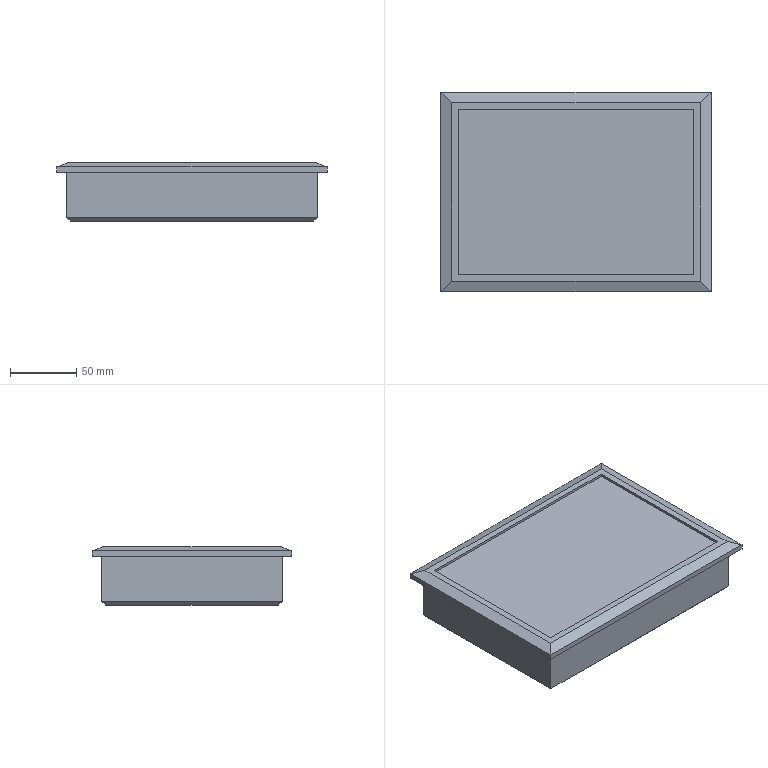Part | STEP file | Xinje TH765 touch screen | 1 solid | 24 faces | box 204 x 150.5 x 44 mm | volume 1119032 mm3 | plane 24
STEP:
#1=CARTESIAN_POINT('',(0.,0.,0.));
#2=DIRECTION('',(0.,0.,1.));
#3=DIRECTION('',(1.,0.,0.));
#4=AXIS2_PLACEMENT_3D('',#1,#2,#3);
#5=CARTESIAN_POINT('',(-43.829,26.896,37.));
#6=VERTEX_POINT('',#5);
#7=CARTESIAN_POINT('',(-43.829,26.896,3.));
#8=VERTEX_POINT('',#7);
#9=CARTESIAN_POINT('',(-43.829,26.896,37.));
#10=DIRECTION('',(0.,0.,-1.));
#11=VECTOR('',#10,1.);
#12=LINE('',#9,#11);
#13=CARTESIAN_POINT('',(-43.829,-109.604,37.));
#14=DIRECTION('',(1.,0.,0.));
#15=DIRECTION('',(0.,0.,-1.));
#16=AXIS2_PLACEMENT_3D('',#13,#14,#15);
#17=PLANE('',#16);
#18=CARTESIAN_POINT('',(0.,136.5));
#19=DIRECTION('',(1.,0.));
#20=VECTOR('',#19,1.);
#21=LINE('',#18,#20);
#22=(GEOMETRIC_REPRESENTATION_CONTEXT(2)PARAMETRIC_REPRESENTATION_CONTEXT()REPRESENTATION_CONTEXT('',''));
#23=DEFINITIONAL_REPRESENTATION('',(#21),#22);
#24=PCURVE('',#17,#23);
#25=CARTESIAN_POINT('',(-43.829,26.896,37.));
#26=DIRECTION('',(0.,-1.,0.));
#27=DIRECTION('',(0.,0.,-1.));
#28=AXIS2_PLACEMENT_3D('',#25,#26,#27);
#29=PLANE('',#28);
#30=CARTESIAN_POINT('',(0.,0.));
#31=DIRECTION('',(1.,0.));
#32=VECTOR('',#31,1.);
#33=LINE('',#30,#32);
#34=(GEOMETRIC_REPRESENTATION_CONTEXT(2)PARAMETRIC_REPRESENTATION_CONTEXT()REPRESENTATION_CONTEXT('',''));
#35=DEFINITIONAL_REPRESENTATION('',(#33),#34);
#36=PCURVE('',#29,#35);
#37=SURFACE_CURVE('',#12,(#24,#36),.PCURVE_S1.);
#38=EDGE_CURVE('',#6,#8,#37,.T.);
#39=ORIENTED_EDGE('',*,*,#38,.T.);
#40=CARTESIAN_POINT('',(-43.829,-109.604,3.));
#41=VERTEX_POINT('',#40);
#42=CARTESIAN_POINT('',(-43.829,-109.604,3.));
#43=DIRECTION('',(0.,-1.,0.));
#44=VECTOR('',#43,1.);
#45=LINE('',#42,#44);
#46=CARTESIAN_POINT('',(34.,0.));
#47=DIRECTION('',(0.,-1.));
#48=VECTOR('',#47,1.);
#49=LINE('',#46,#48);
#50=(GEOMETRIC_REPRESENTATION_CONTEXT(2)PARAMETRIC_REPRESENTATION_CONTEXT()REPRESENTATION_CONTEXT('',''));
#51=DEFINITIONAL_REPRESENTATION('',(#49),#50);
#52=PCURVE('',#17,#51);
#53=CARTESIAN_POINT('',(-43.829,-109.604,3.));
#54=DIRECTION('',(-0.7071,0.,-0.7071));
#55=DIRECTION('',(0.,1.,0.));
#56=AXIS2_PLACEMENT_3D('',#53,#54,#55);
#57=PLANE('',#56);
#58=CARTESIAN_POINT('',(0.,0.));
#59=DIRECTION('',(-1.,0.));
#60=VECTOR('',#59,1.);
#61=LINE('',#58,#60);
#62=(GEOMETRIC_REPRESENTATION_CONTEXT(2)PARAMETRIC_REPRESENTATION_CONTEXT()REPRESENTATION_CONTEXT('',''));
#63=DEFINITIONAL_REPRESENTATION('',(#61),#62);
#64=PCURVE('',#57,#63);
#65=SURFACE_CURVE('',#45,(#52,#64),.PCURVE_S1.);
#66=EDGE_CURVE('',#8,#41,#65,.T.);
#67=ORIENTED_EDGE('',*,*,#66,.T.);
#68=CARTESIAN_POINT('',(-43.829,-109.604,37.));
#69=VERTEX_POINT('',#68);
#70=CARTESIAN_POINT('',(-43.829,-109.604,37.));
#71=DIRECTION('',(0.,0.,-1.));
#72=VECTOR('',#71,1.);
#73=LINE('',#70,#72);
#74=CARTESIAN_POINT('',(0.,0.));
#75=DIRECTION('',(1.,0.));
#76=VECTOR('',#75,1.);
#77=LINE('',#74,#76);
#78=(GEOMETRIC_REPRESENTATION_CONTEXT(2)PARAMETRIC_REPRESENTATION_CONTEXT()REPRESENTATION_CONTEXT('',''));
#79=DEFINITIONAL_REPRESENTATION('',(#77),#78);
#80=PCURVE('',#17,#79);
#81=CARTESIAN_POINT('',(-43.829,-109.604,37.));
#82=DIRECTION('',(0.,1.,0.));
#83=DIRECTION('',(0.,0.,1.));
#84=AXIS2_PLACEMENT_3D('',#81,#82,#83);
#85=PLANE('',#84);
#86=CARTESIAN_POINT('',(0.,0.));
#87=DIRECTION('',(-1.,0.));
#88=VECTOR('',#87,1.);
#89=LINE('',#86,#88);
#90=(GEOMETRIC_REPRESENTATION_CONTEXT(2)PARAMETRIC_REPRESENTATION_CONTEXT()REPRESENTATION_CONTEXT('',''));
#91=DEFINITIONAL_REPRESENTATION('',(#89),#90);
#92=PCURVE('',#85,#91);
#93=SURFACE_CURVE('',#73,(#80,#92),.PCURVE_S1.);
#94=EDGE_CURVE('',#69,#41,#93,.T.);
#95=ORIENTED_EDGE('',*,*,#94,.F.);
#96=CARTESIAN_POINT('',(-43.829,-109.604,37.));
#97=DIRECTION('',(0.,-1.,0.));
#98=VECTOR('',#97,1.);
#99=LINE('',#96,#98);
#100=CARTESIAN_POINT('',(0.,0.));
#101=DIRECTION('',(0.,-1.));
#102=VECTOR('',#101,1.);
#103=LINE('',#100,#102);
#104=(GEOMETRIC_REPRESENTATION_CONTEXT(2)PARAMETRIC_REPRESENTATION_CONTEXT()REPRESENTATION_CONTEXT('',''));
#105=DEFINITIONAL_REPRESENTATION('',(#103),#104);
#106=PCURVE('',#17,#105);
#107=CARTESIAN_POINT('',(0.,0.,37.));
#108=DIRECTION('',(0.,0.,-1.));
#109=DIRECTION('',(-1.,0.,0.));
#110=AXIS2_PLACEMENT_3D('',#107,#108,#109);
#111=PLANE('',#110);
#112=CARTESIAN_POINT('',(43.829,-109.604));
#113=DIRECTION('',(0.,-1.));
#114=VECTOR('',#113,1.);
#115=LINE('',#112,#114);
#116=(GEOMETRIC_REPRESENTATION_CONTEXT(2)PARAMETRIC_REPRESENTATION_CONTEXT()REPRESENTATION_CONTEXT('',''));
#117=DEFINITIONAL_REPRESENTATION('',(#115),#116);
#118=PCURVE('',#111,#117);
#119=SURFACE_CURVE('',#99,(#106,#118),.PCURVE_S1.);
#120=EDGE_CURVE('',#6,#69,#119,.T.);
#121=ORIENTED_EDGE('',*,*,#120,.F.);
#122=EDGE_LOOP('',(#39,#67,#95,#121));
#123=FACE_BOUND('',#122,.T.);
#124=ADVANCED_FACE('',(#123),#17,.F.);
#125=ORIENTED_EDGE('',*,*,#94,.T.);
#126=CARTESIAN_POINT('',(146.171,-109.604,3.));
#127=VERTEX_POINT('',#126);
#128=CARTESIAN_POINT('',(146.171,-109.604,3.));
#129=DIRECTION('',(1.,0.,0.));
#130=VECTOR('',#129,1.);
#131=LINE('',#128,#130);
#132=CARTESIAN_POINT('',(-34.,190.));
#133=DIRECTION('',(0.,1.));
#134=VECTOR('',#133,1.);
#135=LINE('',#132,#134);
#136=(GEOMETRIC_REPRESENTATION_CONTEXT(2)PARAMETRIC_REPRESENTATION_CONTEXT()REPRESENTATION_CONTEXT('',''));
#137=DEFINITIONAL_REPRESENTATION('',(#135),#136);
#138=PCURVE('',#85,#137);
#139=CARTESIAN_POINT('',(-43.829,-109.604,3.));
#140=DIRECTION('',(0.,-0.7071,-0.7071));
#141=DIRECTION('',(-1.,0.,0.));
#142=AXIS2_PLACEMENT_3D('',#139,#140,#141);
#143=PLANE('',#142);
#144=CARTESIAN_POINT('',(-190.,0.));
#145=DIRECTION('',(-1.,0.));
#146=VECTOR('',#145,1.);
#147=LINE('',#144,#146);
#148=(GEOMETRIC_REPRESENTATION_CONTEXT(2)PARAMETRIC_REPRESENTATION_CONTEXT()REPRESENTATION_CONTEXT('',''));
#149=DEFINITIONAL_REPRESENTATION('',(#147),#148);
#150=PCURVE('',#143,#149);
#151=SURFACE_CURVE('',#131,(#138,#150),.PCURVE_S1.);
#152=EDGE_CURVE('',#41,#127,#151,.T.);
#153=ORIENTED_EDGE('',*,*,#152,.T.);
#154=CARTESIAN_POINT('',(146.171,-109.604,37.));
#155=VERTEX_POINT('',#154);
#156=CARTESIAN_POINT('',(146.171,-109.604,37.));
#157=DIRECTION('',(0.,0.,-1.));
#158=VECTOR('',#157,1.);
#159=LINE('',#156,#158);
#160=CARTESIAN_POINT('',(0.,190.));
#161=DIRECTION('',(-1.,0.));
#162=VECTOR('',#161,1.);
#163=LINE('',#160,#162);
#164=(GEOMETRIC_REPRESENTATION_CONTEXT(2)PARAMETRIC_REPRESENTATION_CONTEXT()REPRESENTATION_CONTEXT('',''));
#165=DEFINITIONAL_REPRESENTATION('',(#163),#164);
#166=PCURVE('',#85,#165);
#167=CARTESIAN_POINT('',(146.171,-109.604,37.));
#168=DIRECTION('',(-1.,0.,0.));
#169=DIRECTION('',(0.,0.,1.));
#170=AXIS2_PLACEMENT_3D('',#167,#168,#169);
#171=PLANE('',#170);
#172=CARTESIAN_POINT('',(0.,0.));
#173=DIRECTION('',(-1.,0.));
#174=VECTOR('',#173,1.);
#175=LINE('',#172,#174);
#176=(GEOMETRIC_REPRESENTATION_CONTEXT(2)PARAMETRIC_REPRESENTATION_CONTEXT()REPRESENTATION_CONTEXT('',''));
#177=DEFINITIONAL_REPRESENTATION('',(#175),#176);
#178=PCURVE('',#171,#177);
#179=SURFACE_CURVE('',#159,(#166,#178),.PCURVE_S1.);
#180=EDGE_CURVE('',#155,#127,#179,.T.);
#181=ORIENTED_EDGE('',*,*,#180,.F.);
#182=CARTESIAN_POINT('',(-43.829,-109.604,37.));
#183=DIRECTION('',(1.,0.,0.));
#184=VECTOR('',#183,1.);
#185=LINE('',#182,#184);
#186=CARTESIAN_POINT('',(0.,0.));
#187=DIRECTION('',(0.,1.));
#188=VECTOR('',#187,1.);
#189=LINE('',#186,#188);
#190=(GEOMETRIC_REPRESENTATION_CONTEXT(2)PARAMETRIC_REPRESENTATION_CONTEXT()REPRESENTATION_CONTEXT('',''));
#191=DEFINITIONAL_REPRESENTATION('',(#189),#190);
#192=PCURVE('',#85,#191);
#193=CARTESIAN_POINT('',(43.829,-109.604));
#194=DIRECTION('',(-1.,0.));
#195=VECTOR('',#194,1.);
#196=LINE('',#193,#195);
#197=(GEOMETRIC_REPRESENTATION_CONTEXT(2)PARAMETRIC_REPRESENTATION_CONTEXT()REPRESENTATION_CONTEXT('',''));
#198=DEFINITIONAL_REPRESENTATION('',(#196),#197);
#199=PCURVE('',#111,#198);
#200=SURFACE_CURVE('',#185,(#192,#199),.PCURVE_S1.);
#201=EDGE_CURVE('',#69,#155,#200,.T.);
#202=ORIENTED_EDGE('',*,*,#201,.F.);
#203=EDGE_LOOP('',(#125,#153,#181,#202));
#204=FACE_BOUND('',#203,.T.);
#205=ADVANCED_FACE('',(#204),#85,.F.);
#206=ORIENTED_EDGE('',*,*,#180,.T.);
#207=CARTESIAN_POINT('',(146.171,26.896,3.));
#208=VERTEX_POINT('',#207);
#209=CARTESIAN_POINT('',(146.171,26.896,3.));
#210=DIRECTION('',(0.,1.,0.));
#211=VECTOR('',#210,1.);
#212=LINE('',#209,#211);
#213=CARTESIAN_POINT('',(-34.,136.5));
#214=DIRECTION('',(0.,1.));
#215=VECTOR('',#214,1.);
#216=LINE('',#213,#215);
#217=(GEOMETRIC_REPRESENTATION_CONTEXT(2)PARAMETRIC_REPRESENTATION_CONTEXT()REPRESENTATION_CONTEXT('',''));
#218=DEFINITIONAL_REPRESENTATION('',(#216),#217);
#219=PCURVE('',#171,#218);
#220=CARTESIAN_POINT('',(146.171,-109.604,3.));
#221=DIRECTION('',(0.7071,0.,-0.7071));
#222=DIRECTION('',(0.,-1.,0.));
#223=AXIS2_PLACEMENT_3D('',#220,#221,#222);
#224=PLANE('',#223);
#225=CARTESIAN_POINT('',(-136.5,0.));
#226=DIRECTION('',(-1.,0.));
#227=VECTOR('',#226,1.);
#228=LINE('',#225,#227);
#229=(GEOMETRIC_REPRESENTATION_CONTEXT(2)PARAMETRIC_REPRESENTATION_CONTEXT()REPRESENTATION_CONTEXT('',''));
#230=DEFINITIONAL_REPRESENTATION('',(#228),#229);
#231=PCURVE('',#224,#230);
#232=SURFACE_CURVE('',#212,(#219,#231),.PCURVE_S1.);
#233=EDGE_CURVE('',#127,#208,#232,.T.);
#234=ORIENTED_EDGE('',*,*,#233,.T.);
#235=CARTESIAN_POINT('',(146.171,26.896,37.));
#236=VERTEX_POINT('',#235);
#237=CARTESIAN_POINT('',(146.171,26.896,37.));
#238=DIRECTION('',(0.,0.,-1.));
#239=VECTOR('',#238,1.);
#240=LINE('',#237,#239);
#241=CARTESIAN_POINT('',(0.,136.5));
#242=DIRECTION('',(-1.,0.));
#243=VECTOR('',#242,1.);
#244=LINE('',#241,#243);
#245=(GEOMETRIC_REPRESENTATION_CONTEXT(2)PARAMETRIC_REPRESENTATION_CONTEXT()REPRESENTATION_CONTEXT('',''));
#246=DEFINITIONAL_REPRESENTATION('',(#244),#245);
#247=PCURVE('',#171,#246);
#248=CARTESIAN_POINT('',(0.,190.));
#249=DIRECTION('',(1.,0.));
#250=VECTOR('',#249,1.);
#251=LINE('',#248,#250);
#252=(GEOMETRIC_REPRESENTATION_CONTEXT(2)PARAMETRIC_REPRESENTATION_CONTEXT()REPRESENTATION_CONTEXT('',''));
#253=DEFINITIONAL_REPRESENTATION('',(#251),#252);
#254=PCURVE('',#29,#253);
#255=SURFACE_CURVE('',#240,(#247,#254),.PCURVE_S1.);
#256=EDGE_CURVE('',#236,#208,#255,.T.);
#257=ORIENTED_EDGE('',*,*,#256,.F.);
#258=CARTESIAN_POINT('',(146.171,-109.604,37.));
#259=DIRECTION('',(0.,1.,0.));
#260=VECTOR('',#259,1.);
#261=LINE('',#258,#260);
#262=CARTESIAN_POINT('',(0.,0.));
#263=DIRECTION('',(0.,1.));
#264=VECTOR('',#263,1.);
#265=LINE('',#262,#264);
#266=(GEOMETRIC_REPRESENTATION_CONTEXT(2)PARAMETRIC_REPRESENTATION_CONTEXT()REPRESENTATION_CONTEXT('',''));
#267=DEFINITIONAL_REPRESENTATION('',(#265),#266);
#268=PCURVE('',#171,#267);
#269=CARTESIAN_POINT('',(-146.171,-109.604));
#270=DIRECTION('',(0.,1.));
#271=VECTOR('',#270,1.);
#272=LINE('',#269,#271);
#273=(GEOMETRIC_REPRESENTATION_CONTEXT(2)PARAMETRIC_REPRESENTATION_CONTEXT()REPRESENTATION_CONTEXT('',''));
#274=DEFINITIONAL_REPRESENTATION('',(#272),#273);
#275=PCURVE('',#111,#274);
#276=SURFACE_CURVE('',#261,(#268,#275),.PCURVE_S1.);
#277=EDGE_CURVE('',#155,#236,#276,.T.);
#278=ORIENTED_EDGE('',*,*,#277,.F.);
#279=EDGE_LOOP('',(#206,#234,#257,#278));
#280=FACE_BOUND('',#279,.T.);
#281=ADVANCED_FACE('',(#280),#171,.F.);
#282=ORIENTED_EDGE('',*,*,#256,.T.);
#283=CARTESIAN_POINT('',(-43.829,26.896,3.));
#284=DIRECTION('',(-1.,0.,0.));
#285=VECTOR('',#284,1.);
#286=LINE('',#283,#285);
#287=CARTESIAN_POINT('',(34.,0.));
#288=DIRECTION('',(0.,-1.));
#289=VECTOR('',#288,1.);
#290=LINE('',#287,#289);
#291=(GEOMETRIC_REPRESENTATION_CONTEXT(2)PARAMETRIC_REPRESENTATION_CONTEXT()REPRESENTATION_CONTEXT('',''));
#292=DEFINITIONAL_REPRESENTATION('',(#290),#291);
#293=PCURVE('',#29,#292);
#294=CARTESIAN_POINT('',(-43.829,26.896,3.));
#295=DIRECTION('',(0.,0.7071,-0.7071));
#296=DIRECTION('',(1.,0.,0.));
#297=AXIS2_PLACEMENT_3D('',#294,#295,#296);
#298=PLANE('',#297);
#299=CARTESIAN_POINT('',(0.,0.));
#300=DIRECTION('',(-1.,0.));
#301=VECTOR('',#300,1.);
#302=LINE('',#299,#301);
#303=(GEOMETRIC_REPRESENTATION_CONTEXT(2)PARAMETRIC_REPRESENTATION_CONTEXT()REPRESENTATION_CONTEXT('',''));
#304=DEFINITIONAL_REPRESENTATION('',(#302),#303);
#305=PCURVE('',#298,#304);
#306=SURFACE_CURVE('',#286,(#293,#305),.PCURVE_S1.);
#307=EDGE_CURVE('',#208,#8,#306,.T.);
#308=ORIENTED_EDGE('',*,*,#307,.T.);
#309=ORIENTED_EDGE('',*,*,#38,.F.);
#310=CARTESIAN_POINT('',(-43.829,26.896,37.));
#311=DIRECTION('',(-1.,0.,0.));
#312=VECTOR('',#311,1.);
#313=LINE('',#310,#312);
#314=CARTESIAN_POINT('',(0.,0.));
#315=DIRECTION('',(0.,-1.));
#316=VECTOR('',#315,1.);
#317=LINE('',#314,#316);
#318=(GEOMETRIC_REPRESENTATION_CONTEXT(2)PARAMETRIC_REPRESENTATION_CONTEXT()REPRESENTATION_CONTEXT('',''));
#319=DEFINITIONAL_REPRESENTATION('',(#317),#318);
#320=PCURVE('',#29,#319);
#321=CARTESIAN_POINT('',(43.829,26.896));
#322=DIRECTION('',(1.,0.));
#323=VECTOR('',#322,1.);
#324=LINE('',#321,#323);
#325=(GEOMETRIC_REPRESENTATION_CONTEXT(2)PARAMETRIC_REPRESENTATION_CONTEXT()REPRESENTATION_CONTEXT('',''));
#326=DEFINITIONAL_REPRESENTATION('',(#324),#325);
#327=PCURVE('',#111,#326);
#328=SURFACE_CURVE('',#313,(#320,#327),.PCURVE_S1.);
#329=EDGE_CURVE('',#236,#6,#328,.T.);
#330=ORIENTED_EDGE('',*,*,#329,.F.);
#331=EDGE_LOOP('',(#282,#308,#309,#330));
#332=FACE_BOUND('',#331,.T.);
#333=ADVANCED_FACE('',(#332),#29,.F.);
#334=CARTESIAN_POINT('',(143.171,23.896,0.));
#335=VERTEX_POINT('',#334);
#336=CARTESIAN_POINT('',(143.171,-106.604,0.));
#337=VERTEX_POINT('',#336);
#338=CARTESIAN_POINT('',(143.171,-109.604,0.));
#339=DIRECTION('',(0.,-1.,0.));
#340=VECTOR('',#339,1.);
#341=LINE('',#338,#340);
#342=CARTESIAN_POINT('',(0.,0.,0.));
#343=DIRECTION('',(0.,0.,-1.));
#344=DIRECTION('',(-1.,0.,0.));
#345=AXIS2_PLACEMENT_3D('',#342,#343,#344);
#346=PLANE('',#345);
#347=CARTESIAN_POINT('',(-143.171,-109.604));
#348=DIRECTION('',(0.,-1.));
#349=VECTOR('',#348,1.);
#350=LINE('',#347,#349);
#351=(GEOMETRIC_REPRESENTATION_CONTEXT(2)PARAMETRIC_REPRESENTATION_CONTEXT()REPRESENTATION_CONTEXT('',''));
#352=DEFINITIONAL_REPRESENTATION('',(#350),#351);
#353=PCURVE('',#346,#352);
#354=CARTESIAN_POINT('',(0.,4.243));
#355=DIRECTION('',(1.,0.));
#356=VECTOR('',#355,1.);
#357=LINE('',#354,#356);
#358=(GEOMETRIC_REPRESENTATION_CONTEXT(2)PARAMETRIC_REPRESENTATION_CONTEXT()REPRESENTATION_CONTEXT('',''));
#359=DEFINITIONAL_REPRESENTATION('',(#357),#358);
#360=PCURVE('',#224,#359);
#361=SURFACE_CURVE('',#341,(#353,#360),.PCURVE_S1.);
#362=EDGE_CURVE('',#335,#337,#361,.T.);
#363=ORIENTED_EDGE('',*,*,#362,.T.);
#364=CARTESIAN_POINT('',(-40.829,-106.604,0.));
#365=VERTEX_POINT('',#364);
#366=CARTESIAN_POINT('',(-43.829,-106.604,0.));
#367=DIRECTION('',(-1.,0.,0.));
#368=VECTOR('',#367,1.);
#369=LINE('',#366,#368);
#370=CARTESIAN_POINT('',(43.829,-106.604));
#371=DIRECTION('',(1.,0.));
#372=VECTOR('',#371,1.);
#373=LINE('',#370,#372);
#374=(GEOMETRIC_REPRESENTATION_CONTEXT(2)PARAMETRIC_REPRESENTATION_CONTEXT()REPRESENTATION_CONTEXT('',''));
#375=DEFINITIONAL_REPRESENTATION('',(#373),#374);
#376=PCURVE('',#346,#375);
#377=CARTESIAN_POINT('',(0.,4.243));
#378=DIRECTION('',(1.,0.));
#379=VECTOR('',#378,1.);
#380=LINE('',#377,#379);
#381=(GEOMETRIC_REPRESENTATION_CONTEXT(2)PARAMETRIC_REPRESENTATION_CONTEXT()REPRESENTATION_CONTEXT('',''));
#382=DEFINITIONAL_REPRESENTATION('',(#380),#381);
#383=PCURVE('',#143,#382);
#384=SURFACE_CURVE('',#369,(#376,#383),.PCURVE_S1.);
#385=EDGE_CURVE('',#337,#365,#384,.T.);
#386=ORIENTED_EDGE('',*,*,#385,.T.);
#387=CARTESIAN_POINT('',(-40.829,23.896,0.));
#388=VERTEX_POINT('',#387);
#389=CARTESIAN_POINT('',(-40.829,26.896,0.));
#390=DIRECTION('',(0.,1.,0.));
#391=VECTOR('',#390,1.);
#392=LINE('',#389,#391);
#393=CARTESIAN_POINT('',(40.829,26.896));
#394=DIRECTION('',(0.,1.));
#395=VECTOR('',#394,1.);
#396=LINE('',#393,#395);
#397=(GEOMETRIC_REPRESENTATION_CONTEXT(2)PARAMETRIC_REPRESENTATION_CONTEXT()REPRESENTATION_CONTEXT('',''));
#398=DEFINITIONAL_REPRESENTATION('',(#396),#397);
#399=PCURVE('',#346,#398);
#400=CARTESIAN_POINT('',(136.5,4.243));
#401=DIRECTION('',(1.,0.));
#402=VECTOR('',#401,1.);
#403=LINE('',#400,#402);
#404=(GEOMETRIC_REPRESENTATION_CONTEXT(2)PARAMETRIC_REPRESENTATION_CONTEXT()REPRESENTATION_CONTEXT('',''));
#405=DEFINITIONAL_REPRESENTATION('',(#403),#404);
#406=PCURVE('',#57,#405);
#407=SURFACE_CURVE('',#392,(#399,#406),.PCURVE_S1.);
#408=EDGE_CURVE('',#365,#388,#407,.T.);
#409=ORIENTED_EDGE('',*,*,#408,.T.);
#410=CARTESIAN_POINT('',(146.171,23.896,0.));
#411=DIRECTION('',(1.,0.,0.));
#412=VECTOR('',#411,1.);
#413=LINE('',#410,#412);
#414=CARTESIAN_POINT('',(-146.171,23.896));
#415=DIRECTION('',(-1.,0.));
#416=VECTOR('',#415,1.);
#417=LINE('',#414,#416);
#418=(GEOMETRIC_REPRESENTATION_CONTEXT(2)PARAMETRIC_REPRESENTATION_CONTEXT()REPRESENTATION_CONTEXT('',''));
#419=DEFINITIONAL_REPRESENTATION('',(#417),#418);
#420=PCURVE('',#346,#419);
#421=CARTESIAN_POINT('',(190.,4.243));
#422=DIRECTION('',(1.,0.));
#423=VECTOR('',#422,1.);
#424=LINE('',#421,#423);
#425=(GEOMETRIC_REPRESENTATION_CONTEXT(2)PARAMETRIC_REPRESENTATION_CONTEXT()REPRESENTATION_CONTEXT('',''));
#426=DEFINITIONAL_REPRESENTATION('',(#424),#425);
#427=PCURVE('',#298,#426);
#428=SURFACE_CURVE('',#413,(#420,#427),.PCURVE_S1.);
#429=EDGE_CURVE('',#388,#335,#428,.T.);
#430=ORIENTED_EDGE('',*,*,#429,.T.);
#431=EDGE_LOOP('',(#363,#386,#409,#430));
#432=FACE_BOUND('',#431,.T.);
#433=ADVANCED_FACE('',(#432),#346,.T.);
#434=CARTESIAN_POINT('',(153.171,33.896,37.));
#435=VERTEX_POINT('',#434);
#436=CARTESIAN_POINT('',(-50.829,33.896,37.));
#437=VERTEX_POINT('',#436);
#438=CARTESIAN_POINT('',(-50.829,33.896,37.));
#439=DIRECTION('',(-1.,0.,0.));
#440=VECTOR('',#439,1.);
#441=LINE('',#438,#440);
#442=CARTESIAN_POINT('',(50.829,33.896));
#443=DIRECTION('',(1.,0.));
#444=VECTOR('',#443,1.);
#445=LINE('',#442,#444);
#446=(GEOMETRIC_REPRESENTATION_CONTEXT(2)PARAMETRIC_REPRESENTATION_CONTEXT()REPRESENTATION_CONTEXT('',''));
#447=DEFINITIONAL_REPRESENTATION('',(#445),#446);
#448=PCURVE('',#111,#447);
#449=CARTESIAN_POINT('',(-50.829,33.896,44.));
#450=DIRECTION('',(0.,-1.,0.));
#451=DIRECTION('',(0.,0.,-1.));
#452=AXIS2_PLACEMENT_3D('',#449,#450,#451);
#453=PLANE('',#452);
#454=CARTESIAN_POINT('',(7.,0.));
#455=DIRECTION('',(0.,-1.));
#456=VECTOR('',#455,1.);
#457=LINE('',#454,#456);
#458=(GEOMETRIC_REPRESENTATION_CONTEXT(2)PARAMETRIC_REPRESENTATION_CONTEXT()REPRESENTATION_CONTEXT('',''));
#459=DEFINITIONAL_REPRESENTATION('',(#457),#458);
#460=PCURVE('',#453,#459);
#461=SURFACE_CURVE('',#441,(#448,#460),.PCURVE_S1.);
#462=EDGE_CURVE('',#435,#437,#461,.T.);
#463=ORIENTED_EDGE('',*,*,#462,.F.);
#464=CARTESIAN_POINT('',(153.171,-116.604,37.));
#465=VERTEX_POINT('',#464);
#466=CARTESIAN_POINT('',(153.171,33.896,37.));
#467=DIRECTION('',(0.,1.,0.));
#468=VECTOR('',#467,1.);
#469=LINE('',#466,#468);
#470=CARTESIAN_POINT('',(-153.171,33.896));
#471=DIRECTION('',(0.,1.));
#472=VECTOR('',#471,1.);
#473=LINE('',#470,#472);
#474=(GEOMETRIC_REPRESENTATION_CONTEXT(2)PARAMETRIC_REPRESENTATION_CONTEXT()REPRESENTATION_CONTEXT('',''));
#475=DEFINITIONAL_REPRESENTATION('',(#473),#474);
#476=PCURVE('',#111,#475);
#477=CARTESIAN_POINT('',(153.171,33.896,44.));
#478=DIRECTION('',(-1.,0.,0.));
#479=DIRECTION('',(0.,0.,1.));
#480=AXIS2_PLACEMENT_3D('',#477,#478,#479);
#481=PLANE('',#480);
#482=CARTESIAN_POINT('',(-7.,0.));
#483=DIRECTION('',(0.,1.));
#484=VECTOR('',#483,1.);
#485=LINE('',#482,#484);
#486=(GEOMETRIC_REPRESENTATION_CONTEXT(2)PARAMETRIC_REPRESENTATION_CONTEXT()REPRESENTATION_CONTEXT('',''));
#487=DEFINITIONAL_REPRESENTATION('',(#485),#486);
#488=PCURVE('',#481,#487);
#489=SURFACE_CURVE('',#469,(#476,#488),.PCURVE_S1.);
#490=EDGE_CURVE('',#465,#435,#489,.T.);
#491=ORIENTED_EDGE('',*,*,#490,.F.);
#492=CARTESIAN_POINT('',(-50.829,-116.604,37.));
#493=VERTEX_POINT('',#492);
#494=CARTESIAN_POINT('',(-50.829,-116.604,37.));
#495=DIRECTION('',(1.,0.,0.));
#496=VECTOR('',#495,1.);
#497=LINE('',#494,#496);
#498=CARTESIAN_POINT('',(50.829,-116.604));
#499=DIRECTION('',(-1.,0.));
#500=VECTOR('',#499,1.);
#501=LINE('',#498,#500);
#502=(GEOMETRIC_REPRESENTATION_CONTEXT(2)PARAMETRIC_REPRESENTATION_CONTEXT()REPRESENTATION_CONTEXT('',''));
#503=DEFINITIONAL_REPRESENTATION('',(#501),#502);
#504=PCURVE('',#111,#503);
#505=CARTESIAN_POINT('',(-50.829,-116.604,44.));
#506=DIRECTION('',(0.,1.,0.));
#507=DIRECTION('',(0.,0.,1.));
#508=AXIS2_PLACEMENT_3D('',#505,#506,#507);
#509=PLANE('',#508);
#510=CARTESIAN_POINT('',(-7.,0.));
#511=DIRECTION('',(0.,1.));
#512=VECTOR('',#511,1.);
#513=LINE('',#510,#512);
#514=(GEOMETRIC_REPRESENTATION_CONTEXT(2)PARAMETRIC_REPRESENTATION_CONTEXT()REPRESENTATION_CONTEXT('',''));
#515=DEFINITIONAL_REPRESENTATION('',(#513),#514);
#516=PCURVE('',#509,#515);
#517=SURFACE_CURVE('',#497,(#504,#516),.PCURVE_S1.);
#518=EDGE_CURVE('',#493,#465,#517,.T.);
#519=ORIENTED_EDGE('',*,*,#518,.F.);
#520=CARTESIAN_POINT('',(-50.829,33.896,37.));
#521=DIRECTION('',(0.,-1.,0.));
#522=VECTOR('',#521,1.);
#523=LINE('',#520,#522);
#524=CARTESIAN_POINT('',(50.829,33.896));
#525=DIRECTION('',(0.,-1.));
#526=VECTOR('',#525,1.);
#527=LINE('',#524,#526);
#528=(GEOMETRIC_REPRESENTATION_CONTEXT(2)PARAMETRIC_REPRESENTATION_CONTEXT()REPRESENTATION_CONTEXT('',''));
#529=DEFINITIONAL_REPRESENTATION('',(#527),#528);
#530=PCURVE('',#111,#529);
#531=CARTESIAN_POINT('',(-50.829,33.896,44.));
#532=DIRECTION('',(1.,0.,0.));
#533=DIRECTION('',(0.,0.,-1.));
#534=AXIS2_PLACEMENT_3D('',#531,#532,#533);
#535=PLANE('',#534);
#536=CARTESIAN_POINT('',(7.,0.));
#537=DIRECTION('',(0.,-1.));
#538=VECTOR('',#537,1.);
#539=LINE('',#536,#538);
#540=(GEOMETRIC_REPRESENTATION_CONTEXT(2)PARAMETRIC_REPRESENTATION_CONTEXT()REPRESENTATION_CONTEXT('',''));
#541=DEFINITIONAL_REPRESENTATION('',(#539),#540);
#542=PCURVE('',#535,#541);
#543=SURFACE_CURVE('',#523,(#530,#542),.PCURVE_S1.);
#544=EDGE_CURVE('',#437,#493,#543,.T.);
#545=ORIENTED_EDGE('',*,*,#544,.F.);
#546=EDGE_LOOP('',(#463,#491,#519,#545));
#547=FACE_BOUND('',#546,.T.);
#548=ORIENTED_EDGE('',*,*,#120,.T.);
#549=ORIENTED_EDGE('',*,*,#201,.T.);
#550=ORIENTED_EDGE('',*,*,#277,.T.);
#551=ORIENTED_EDGE('',*,*,#329,.T.);
#552=EDGE_LOOP('',(#548,#549,#550,#551));
#553=FACE_BOUND('',#552,.T.);
#554=ADVANCED_FACE('',(#547,#553),#111,.T.);
#555=CARTESIAN_POINT('',(-50.829,33.896,41.));
#556=VERTEX_POINT('',#555);
#557=CARTESIAN_POINT('',(-50.829,33.896,44.));
#558=DIRECTION('',(0.,0.,-1.));
#559=VECTOR('',#558,1.);
#560=LINE('',#557,#559);
#561=CARTESIAN_POINT('',(0.,0.));
#562=DIRECTION('',(1.,0.));
#563=VECTOR('',#562,1.);
#564=LINE('',#561,#563);
#565=(GEOMETRIC_REPRESENTATION_CONTEXT(2)PARAMETRIC_REPRESENTATION_CONTEXT()REPRESENTATION_CONTEXT('',''));
#566=DEFINITIONAL_REPRESENTATION('',(#564),#565);
#567=PCURVE('',#453,#566);
#568=CARTESIAN_POINT('',(0.,0.));
#569=DIRECTION('',(1.,0.));
#570=VECTOR('',#569,1.);
#571=LINE('',#568,#570);
#572=(GEOMETRIC_REPRESENTATION_CONTEXT(2)PARAMETRIC_REPRESENTATION_CONTEXT()REPRESENTATION_CONTEXT('',''));
#573=DEFINITIONAL_REPRESENTATION('',(#571),#572);
#574=PCURVE('',#535,#573);
#575=SURFACE_CURVE('',#560,(#567,#574),.PCURVE_S1.);
#576=EDGE_CURVE('',#556,#437,#575,.T.);
#577=ORIENTED_EDGE('',*,*,#576,.F.);
#578=CARTESIAN_POINT('',(153.171,33.896,41.));
#579=VERTEX_POINT('',#578);
#580=CARTESIAN_POINT('',(-50.829,33.896,41.));
#581=DIRECTION('',(1.,0.,0.));
#582=VECTOR('',#581,1.);
#583=LINE('',#580,#582);
#584=CARTESIAN_POINT('',(3.,0.));
#585=DIRECTION('',(0.,1.));
#586=VECTOR('',#585,1.);
#587=LINE('',#584,#586);
#588=(GEOMETRIC_REPRESENTATION_CONTEXT(2)PARAMETRIC_REPRESENTATION_CONTEXT()REPRESENTATION_CONTEXT('',''));
#589=DEFINITIONAL_REPRESENTATION('',(#587),#588);
#590=PCURVE('',#453,#589);
#591=CARTESIAN_POINT('',(0.,25.896,44.));
#592=DIRECTION('',(0.,-0.3511,-0.9363));
#593=DIRECTION('',(-1.,0.,0.));
#594=AXIS2_PLACEMENT_3D('',#591,#592,#593);
#595=PLANE('',#594);
#596=CARTESIAN_POINT('',(50.829,8.544));
#597=DIRECTION('',(-1.,0.));
#598=VECTOR('',#597,1.);
#599=LINE('',#596,#598);
#600=(GEOMETRIC_REPRESENTATION_CONTEXT(2)PARAMETRIC_REPRESENTATION_CONTEXT()REPRESENTATION_CONTEXT('',''));
#601=DEFINITIONAL_REPRESENTATION('',(#599),#600);
#602=PCURVE('',#595,#601);
#603=SURFACE_CURVE('',#583,(#590,#602),.PCURVE_S1.);
#604=EDGE_CURVE('',#556,#579,#603,.T.);
#605=ORIENTED_EDGE('',*,*,#604,.T.);
#606=CARTESIAN_POINT('',(153.171,33.896,44.));
#607=DIRECTION('',(0.,0.,-1.));
#608=VECTOR('',#607,1.);
#609=LINE('',#606,#608);
#610=CARTESIAN_POINT('',(0.,204.));
#611=DIRECTION('',(1.,0.));
#612=VECTOR('',#611,1.);
#613=LINE('',#610,#612);
#614=(GEOMETRIC_REPRESENTATION_CONTEXT(2)PARAMETRIC_REPRESENTATION_CONTEXT()REPRESENTATION_CONTEXT('',''));
#615=DEFINITIONAL_REPRESENTATION('',(#613),#614);
#616=PCURVE('',#453,#615);
#617=CARTESIAN_POINT('',(0.,0.));
#618=DIRECTION('',(-1.,0.));
#619=VECTOR('',#618,1.);
#620=LINE('',#617,#619);
#621=(GEOMETRIC_REPRESENTATION_CONTEXT(2)PARAMETRIC_REPRESENTATION_CONTEXT()REPRESENTATION_CONTEXT('',''));
#622=DEFINITIONAL_REPRESENTATION('',(#620),#621);
#623=PCURVE('',#481,#622);
#624=SURFACE_CURVE('',#609,(#616,#623),.PCURVE_S1.);
#625=EDGE_CURVE('',#579,#435,#624,.T.);
#626=ORIENTED_EDGE('',*,*,#625,.T.);
#627=ORIENTED_EDGE('',*,*,#462,.T.);
#628=EDGE_LOOP('',(#577,#605,#626,#627));
#629=FACE_BOUND('',#628,.T.);
#630=ADVANCED_FACE('',(#629),#453,.F.);
#631=CARTESIAN_POINT('',(-50.829,-116.604,41.));
#632=VERTEX_POINT('',#631);
#633=CARTESIAN_POINT('',(-50.829,-116.604,44.));
#634=DIRECTION('',(0.,0.,-1.));
#635=VECTOR('',#634,1.);
#636=LINE('',#633,#635);
#637=CARTESIAN_POINT('',(0.,-150.5));
#638=DIRECTION('',(1.,0.));
#639=VECTOR('',#638,1.);
#640=LINE('',#637,#639);
#641=(GEOMETRIC_REPRESENTATION_CONTEXT(2)PARAMETRIC_REPRESENTATION_CONTEXT()REPRESENTATION_CONTEXT('',''));
#642=DEFINITIONAL_REPRESENTATION('',(#640),#641);
#643=PCURVE('',#535,#642);
#644=CARTESIAN_POINT('',(0.,0.));
#645=DIRECTION('',(-1.,0.));
#646=VECTOR('',#645,1.);
#647=LINE('',#644,#646);
#648=(GEOMETRIC_REPRESENTATION_CONTEXT(2)PARAMETRIC_REPRESENTATION_CONTEXT()REPRESENTATION_CONTEXT('',''));
#649=DEFINITIONAL_REPRESENTATION('',(#647),#648);
#650=PCURVE('',#509,#649);
#651=SURFACE_CURVE('',#636,(#643,#650),.PCURVE_S1.);
#652=EDGE_CURVE('',#632,#493,#651,.T.);
#653=ORIENTED_EDGE('',*,*,#652,.F.);
#654=CARTESIAN_POINT('',(-50.829,33.896,41.));
#655=DIRECTION('',(0.,1.,0.));
#656=VECTOR('',#655,1.);
#657=LINE('',#654,#656);
#658=CARTESIAN_POINT('',(3.,0.));
#659=DIRECTION('',(0.,1.));
#660=VECTOR('',#659,1.);
#661=LINE('',#658,#660);
#662=(GEOMETRIC_REPRESENTATION_CONTEXT(2)PARAMETRIC_REPRESENTATION_CONTEXT()REPRESENTATION_CONTEXT('',''));
#663=DEFINITIONAL_REPRESENTATION('',(#661),#662);
#664=PCURVE('',#535,#663);
#665=CARTESIAN_POINT('',(-42.829,0.,44.));
#666=DIRECTION('',(0.3511,0.,-0.9363));
#667=DIRECTION('',(0.,-1.,0.));
#668=AXIS2_PLACEMENT_3D('',#665,#666,#667);
#669=PLANE('',#668);
#670=CARTESIAN_POINT('',(-33.896,8.544));
#671=DIRECTION('',(-1.,0.));
#672=VECTOR('',#671,1.);
#673=LINE('',#670,#672);
#674=(GEOMETRIC_REPRESENTATION_CONTEXT(2)PARAMETRIC_REPRESENTATION_CONTEXT()REPRESENTATION_CONTEXT('',''));
#675=DEFINITIONAL_REPRESENTATION('',(#673),#674);
#676=PCURVE('',#669,#675);
#677=SURFACE_CURVE('',#657,(#664,#676),.PCURVE_S1.);
#678=EDGE_CURVE('',#632,#556,#677,.T.);
#679=ORIENTED_EDGE('',*,*,#678,.T.);
#680=ORIENTED_EDGE('',*,*,#576,.T.);
#681=ORIENTED_EDGE('',*,*,#544,.T.);
#682=EDGE_LOOP('',(#653,#679,#680,#681));
#683=FACE_BOUND('',#682,.T.);
#684=ADVANCED_FACE('',(#683),#535,.F.);
#685=CARTESIAN_POINT('',(153.171,-116.604,41.));
#686=VERTEX_POINT('',#685);
#687=CARTESIAN_POINT('',(153.171,-116.604,44.));
#688=DIRECTION('',(0.,0.,-1.));
#689=VECTOR('',#688,1.);
#690=LINE('',#687,#689);
#691=CARTESIAN_POINT('',(0.,204.));
#692=DIRECTION('',(-1.,0.));
#693=VECTOR('',#692,1.);
#694=LINE('',#691,#693);
#695=(GEOMETRIC_REPRESENTATION_CONTEXT(2)PARAMETRIC_REPRESENTATION_CONTEXT()REPRESENTATION_CONTEXT('',''));
#696=DEFINITIONAL_REPRESENTATION('',(#694),#695);
#697=PCURVE('',#509,#696);
#698=CARTESIAN_POINT('',(0.,-150.5));
#699=DIRECTION('',(-1.,0.));
#700=VECTOR('',#699,1.);
#701=LINE('',#698,#700);
#702=(GEOMETRIC_REPRESENTATION_CONTEXT(2)PARAMETRIC_REPRESENTATION_CONTEXT()REPRESENTATION_CONTEXT('',''));
#703=DEFINITIONAL_REPRESENTATION('',(#701),#702);
#704=PCURVE('',#481,#703);
#705=SURFACE_CURVE('',#690,(#697,#704),.PCURVE_S1.);
#706=EDGE_CURVE('',#686,#465,#705,.T.);
#707=ORIENTED_EDGE('',*,*,#706,.F.);
#708=CARTESIAN_POINT('',(-50.829,-116.604,41.));
#709=DIRECTION('',(-1.,0.,0.));
#710=VECTOR('',#709,1.);
#711=LINE('',#708,#710);
#712=CARTESIAN_POINT('',(-3.,0.));
#713=DIRECTION('',(0.,-1.));
#714=VECTOR('',#713,1.);
#715=LINE('',#712,#714);
#716=(GEOMETRIC_REPRESENTATION_CONTEXT(2)PARAMETRIC_REPRESENTATION_CONTEXT()REPRESENTATION_CONTEXT('',''));
#717=DEFINITIONAL_REPRESENTATION('',(#715),#716);
#718=PCURVE('',#509,#717);
#719=CARTESIAN_POINT('',(0.,-108.604,44.));
#720=DIRECTION('',(0.,0.3511,-0.9363));
#721=DIRECTION('',(1.,0.,0.));
#722=AXIS2_PLACEMENT_3D('',#719,#720,#721);
#723=PLANE('',#722);
#724=CARTESIAN_POINT('',(-50.829,8.544));
#725=DIRECTION('',(-1.,0.));
#726=VECTOR('',#725,1.);
#727=LINE('',#724,#726);
#728=(GEOMETRIC_REPRESENTATION_CONTEXT(2)PARAMETRIC_REPRESENTATION_CONTEXT()REPRESENTATION_CONTEXT('',''));
#729=DEFINITIONAL_REPRESENTATION('',(#727),#728);
#730=PCURVE('',#723,#729);
#731=SURFACE_CURVE('',#711,(#718,#730),.PCURVE_S1.);
#732=EDGE_CURVE('',#686,#632,#731,.T.);
#733=ORIENTED_EDGE('',*,*,#732,.T.);
#734=ORIENTED_EDGE('',*,*,#652,.T.);
#735=ORIENTED_EDGE('',*,*,#518,.T.);
#736=EDGE_LOOP('',(#707,#733,#734,#735));
#737=FACE_BOUND('',#736,.T.);
#738=ADVANCED_FACE('',(#737),#509,.F.);
#739=ORIENTED_EDGE('',*,*,#625,.F.);
#740=CARTESIAN_POINT('',(153.171,33.896,41.));
#741=DIRECTION('',(0.,-1.,0.));
#742=VECTOR('',#741,1.);
#743=LINE('',#740,#742);
#744=CARTESIAN_POINT('',(-3.,0.));
#745=DIRECTION('',(0.,-1.));
#746=VECTOR('',#745,1.);
#747=LINE('',#744,#746);
#748=(GEOMETRIC_REPRESENTATION_CONTEXT(2)PARAMETRIC_REPRESENTATION_CONTEXT()REPRESENTATION_CONTEXT('',''));
#749=DEFINITIONAL_REPRESENTATION('',(#747),#748);
#750=PCURVE('',#481,#749);
#751=CARTESIAN_POINT('',(145.171,0.,44.));
#752=DIRECTION('',(-0.3511,0.,-0.9363));
#753=DIRECTION('',(0.,1.,0.));
#754=AXIS2_PLACEMENT_3D('',#751,#752,#753);
#755=PLANE('',#754);
#756=CARTESIAN_POINT('',(33.896,8.544));
#757=DIRECTION('',(-1.,0.));
#758=VECTOR('',#757,1.);
#759=LINE('',#756,#758);
#760=(GEOMETRIC_REPRESENTATION_CONTEXT(2)PARAMETRIC_REPRESENTATION_CONTEXT()REPRESENTATION_CONTEXT('',''));
#761=DEFINITIONAL_REPRESENTATION('',(#759),#760);
#762=PCURVE('',#755,#761);
#763=SURFACE_CURVE('',#743,(#750,#762),.PCURVE_S1.);
#764=EDGE_CURVE('',#579,#686,#763,.T.);
#765=ORIENTED_EDGE('',*,*,#764,.T.);
#766=ORIENTED_EDGE('',*,*,#706,.T.);
#767=ORIENTED_EDGE('',*,*,#490,.T.);
#768=EDGE_LOOP('',(#739,#765,#766,#767));
#769=FACE_BOUND('',#768,.T.);
#770=ADVANCED_FACE('',(#769),#481,.F.);
#771=CARTESIAN_POINT('',(-37.829,-103.604,44.));
#772=VERTEX_POINT('',#771);
#773=CARTESIAN_POINT('',(140.171,-103.604,44.));
#774=VERTEX_POINT('',#773);
#775=CARTESIAN_POINT('',(-37.829,-103.604,44.));
#776=DIRECTION('',(1.,0.,0.));
#777=VECTOR('',#776,1.);
#778=LINE('',#775,#777);
#779=CARTESIAN_POINT('',(0.,0.,44.));
#780=DIRECTION('',(0.,0.,-1.));
#781=DIRECTION('',(-1.,0.,0.));
#782=AXIS2_PLACEMENT_3D('',#779,#780,#781);
#783=PLANE('',#782);
#784=CARTESIAN_POINT('',(37.829,-103.604));
#785=DIRECTION('',(-1.,0.));
#786=VECTOR('',#785,1.);
#787=LINE('',#784,#786);
#788=(GEOMETRIC_REPRESENTATION_CONTEXT(2)PARAMETRIC_REPRESENTATION_CONTEXT()REPRESENTATION_CONTEXT('',''));
#789=DEFINITIONAL_REPRESENTATION('',(#787),#788);
#790=PCURVE('',#783,#789);
#791=CARTESIAN_POINT('',(-37.829,-103.604,42.));
#792=DIRECTION('',(0.,-1.,0.));
#793=DIRECTION('',(1.,0.,0.));
#794=AXIS2_PLACEMENT_3D('',#791,#792,#793);
#795=PLANE('',#794);
#796=CARTESIAN_POINT('',(0.,2.));
#797=DIRECTION('',(1.,0.));
#798=VECTOR('',#797,1.);
#799=LINE('',#796,#798);
#800=(GEOMETRIC_REPRESENTATION_CONTEXT(2)PARAMETRIC_REPRESENTATION_CONTEXT()REPRESENTATION_CONTEXT('',''));
#801=DEFINITIONAL_REPRESENTATION('',(#799),#800);
#802=PCURVE('',#795,#801);
#803=SURFACE_CURVE('',#778,(#790,#802),.PCURVE_S1.);
#804=EDGE_CURVE('',#772,#774,#803,.T.);
#805=ORIENTED_EDGE('',*,*,#804,.F.);
#806=CARTESIAN_POINT('',(-37.829,20.896,44.));
#807=VERTEX_POINT('',#806);
#808=CARTESIAN_POINT('',(-37.829,20.896,44.));
#809=DIRECTION('',(0.,-1.,0.));
#810=VECTOR('',#809,1.);
#811=LINE('',#808,#810);
#812=CARTESIAN_POINT('',(37.829,20.896));
#813=DIRECTION('',(0.,-1.));
#814=VECTOR('',#813,1.);
#815=LINE('',#812,#814);
#816=(GEOMETRIC_REPRESENTATION_CONTEXT(2)PARAMETRIC_REPRESENTATION_CONTEXT()REPRESENTATION_CONTEXT('',''));
#817=DEFINITIONAL_REPRESENTATION('',(#815),#816);
#818=PCURVE('',#783,#817);
#819=CARTESIAN_POINT('',(-37.829,20.896,42.));
#820=DIRECTION('',(-1.,0.,0.));
#821=DIRECTION('',(0.,0.,1.));
#822=AXIS2_PLACEMENT_3D('',#819,#820,#821);
#823=PLANE('',#822);
#824=CARTESIAN_POINT('',(2.,0.));
#825=DIRECTION('',(0.,-1.));
#826=VECTOR('',#825,1.);
#827=LINE('',#824,#826);
#828=(GEOMETRIC_REPRESENTATION_CONTEXT(2)PARAMETRIC_REPRESENTATION_CONTEXT()REPRESENTATION_CONTEXT('',''));
#829=DEFINITIONAL_REPRESENTATION('',(#827),#828);
#830=PCURVE('',#823,#829);
#831=SURFACE_CURVE('',#811,(#818,#830),.PCURVE_S1.);
#832=EDGE_CURVE('',#807,#772,#831,.T.);
#833=ORIENTED_EDGE('',*,*,#832,.F.);
#834=CARTESIAN_POINT('',(140.171,20.896,44.));
#835=VERTEX_POINT('',#834);
#836=CARTESIAN_POINT('',(-37.829,20.896,44.));
#837=DIRECTION('',(-1.,0.,0.));
#838=VECTOR('',#837,1.);
#839=LINE('',#836,#838);
#840=CARTESIAN_POINT('',(37.829,20.896));
#841=DIRECTION('',(1.,0.));
#842=VECTOR('',#841,1.);
#843=LINE('',#840,#842);
#844=(GEOMETRIC_REPRESENTATION_CONTEXT(2)PARAMETRIC_REPRESENTATION_CONTEXT()REPRESENTATION_CONTEXT('',''));
#845=DEFINITIONAL_REPRESENTATION('',(#843),#844);
#846=PCURVE('',#783,#845);
#847=CARTESIAN_POINT('',(-37.829,20.896,42.));
#848=DIRECTION('',(0.,1.,0.));
#849=DIRECTION('',(0.,0.,1.));
#850=AXIS2_PLACEMENT_3D('',#847,#848,#849);
#851=PLANE('',#850);
#852=CARTESIAN_POINT('',(2.,0.));
#853=DIRECTION('',(0.,-1.));
#854=VECTOR('',#853,1.);
#855=LINE('',#852,#854);
#856=(GEOMETRIC_REPRESENTATION_CONTEXT(2)PARAMETRIC_REPRESENTATION_CONTEXT()REPRESENTATION_CONTEXT('',''));
#857=DEFINITIONAL_REPRESENTATION('',(#855),#856);
#858=PCURVE('',#851,#857);
#859=SURFACE_CURVE('',#839,(#846,#858),.PCURVE_S1.);
#860=EDGE_CURVE('',#835,#807,#859,.T.);
#861=ORIENTED_EDGE('',*,*,#860,.F.);
#862=CARTESIAN_POINT('',(140.171,20.896,44.));
#863=DIRECTION('',(0.,1.,0.));
#864=VECTOR('',#863,1.);
#865=LINE('',#862,#864);
#866=CARTESIAN_POINT('',(-140.171,20.896));
#867=DIRECTION('',(0.,1.));
#868=VECTOR('',#867,1.);
#869=LINE('',#866,#868);
#870=(GEOMETRIC_REPRESENTATION_CONTEXT(2)PARAMETRIC_REPRESENTATION_CONTEXT()REPRESENTATION_CONTEXT('',''));
#871=DEFINITIONAL_REPRESENTATION('',(#869),#870);
#872=PCURVE('',#783,#871);
#873=CARTESIAN_POINT('',(140.171,20.896,42.));
#874=DIRECTION('',(1.,0.,0.));
#875=DIRECTION('',(0.,0.,-1.));
#876=AXIS2_PLACEMENT_3D('',#873,#874,#875);
#877=PLANE('',#876);
#878=CARTESIAN_POINT('',(-2.,0.));
#879=DIRECTION('',(0.,1.));
#880=VECTOR('',#879,1.);
#881=LINE('',#878,#880);
#882=(GEOMETRIC_REPRESENTATION_CONTEXT(2)PARAMETRIC_REPRESENTATION_CONTEXT()REPRESENTATION_CONTEXT('',''));
#883=DEFINITIONAL_REPRESENTATION('',(#881),#882);
#884=PCURVE('',#877,#883);
#885=SURFACE_CURVE('',#865,(#872,#884),.PCURVE_S1.);
#886=EDGE_CURVE('',#774,#835,#885,.T.);
#887=ORIENTED_EDGE('',*,*,#886,.F.);
#888=EDGE_LOOP('',(#805,#833,#861,#887));
#889=FACE_BOUND('',#888,.T.);
#890=CARTESIAN_POINT('',(-42.829,-108.604,44.));
#891=VERTEX_POINT('',#890);
#892=CARTESIAN_POINT('',(145.171,-108.604,44.));
#893=VERTEX_POINT('',#892);
#894=CARTESIAN_POINT('',(0.,-108.604,44.));
#895=DIRECTION('',(1.,0.,0.));
#896=VECTOR('',#895,1.);
#897=LINE('',#894,#896);
#898=CARTESIAN_POINT('',(0.,-108.604));
#899=DIRECTION('',(-1.,0.));
#900=VECTOR('',#899,1.);
#901=LINE('',#898,#900);
#902=(GEOMETRIC_REPRESENTATION_CONTEXT(2)PARAMETRIC_REPRESENTATION_CONTEXT()REPRESENTATION_CONTEXT('',''));
#903=DEFINITIONAL_REPRESENTATION('',(#901),#902);
#904=PCURVE('',#783,#903);
#905=CARTESIAN_POINT('',(0.,0.));
#906=DIRECTION('',(1.,0.));
#907=VECTOR('',#906,1.);
#908=LINE('',#905,#907);
#909=(GEOMETRIC_REPRESENTATION_CONTEXT(2)PARAMETRIC_REPRESENTATION_CONTEXT()REPRESENTATION_CONTEXT('',''));
#910=DEFINITIONAL_REPRESENTATION('',(#908),#909);
#911=PCURVE('',#723,#910);
#912=SURFACE_CURVE('',#897,(#904,#911),.PCURVE_S1.);
#913=EDGE_CURVE('',#891,#893,#912,.T.);
#914=ORIENTED_EDGE('',*,*,#913,.T.);
#915=CARTESIAN_POINT('',(145.171,25.896,44.));
#916=VERTEX_POINT('',#915);
#917=CARTESIAN_POINT('',(145.171,0.,44.));
#918=DIRECTION('',(0.,1.,0.));
#919=VECTOR('',#918,1.);
#920=LINE('',#917,#919);
#921=CARTESIAN_POINT('',(-145.171,0.));
#922=DIRECTION('',(0.,1.));
#923=VECTOR('',#922,1.);
#924=LINE('',#921,#923);
#925=(GEOMETRIC_REPRESENTATION_CONTEXT(2)PARAMETRIC_REPRESENTATION_CONTEXT()REPRESENTATION_CONTEXT('',''));
#926=DEFINITIONAL_REPRESENTATION('',(#924),#925);
#927=PCURVE('',#783,#926);
#928=CARTESIAN_POINT('',(0.,0.));
#929=DIRECTION('',(1.,0.));
#930=VECTOR('',#929,1.);
#931=LINE('',#928,#930);
#932=(GEOMETRIC_REPRESENTATION_CONTEXT(2)PARAMETRIC_REPRESENTATION_CONTEXT()REPRESENTATION_CONTEXT('',''));
#933=DEFINITIONAL_REPRESENTATION('',(#931),#932);
#934=PCURVE('',#755,#933);
#935=SURFACE_CURVE('',#920,(#927,#934),.PCURVE_S1.);
#936=EDGE_CURVE('',#893,#916,#935,.T.);
#937=ORIENTED_EDGE('',*,*,#936,.T.);
#938=CARTESIAN_POINT('',(-42.829,25.896,44.));
#939=VERTEX_POINT('',#938);
#940=CARTESIAN_POINT('',(0.,25.896,44.));
#941=DIRECTION('',(-1.,0.,0.));
#942=VECTOR('',#941,1.);
#943=LINE('',#940,#942);
#944=CARTESIAN_POINT('',(0.,25.896));
#945=DIRECTION('',(1.,0.));
#946=VECTOR('',#945,1.);
#947=LINE('',#944,#946);
#948=(GEOMETRIC_REPRESENTATION_CONTEXT(2)PARAMETRIC_REPRESENTATION_CONTEXT()REPRESENTATION_CONTEXT('',''));
#949=DEFINITIONAL_REPRESENTATION('',(#947),#948);
#950=PCURVE('',#783,#949);
#951=CARTESIAN_POINT('',(0.,0.));
#952=DIRECTION('',(1.,0.));
#953=VECTOR('',#952,1.);
#954=LINE('',#951,#953);
#955=(GEOMETRIC_REPRESENTATION_CONTEXT(2)PARAMETRIC_REPRESENTATION_CONTEXT()REPRESENTATION_CONTEXT('',''));
#956=DEFINITIONAL_REPRESENTATION('',(#954),#955);
#957=PCURVE('',#595,#956);
#958=SURFACE_CURVE('',#943,(#950,#957),.PCURVE_S1.);
#959=EDGE_CURVE('',#916,#939,#958,.T.);
#960=ORIENTED_EDGE('',*,*,#959,.T.);
#961=CARTESIAN_POINT('',(-42.829,0.,44.));
#962=DIRECTION('',(0.,-1.,0.));
#963=VECTOR('',#962,1.);
#964=LINE('',#961,#963);
#965=CARTESIAN_POINT('',(42.829,0.));
#966=DIRECTION('',(0.,-1.));
#967=VECTOR('',#966,1.);
#968=LINE('',#965,#967);
#969=(GEOMETRIC_REPRESENTATION_CONTEXT(2)PARAMETRIC_REPRESENTATION_CONTEXT()REPRESENTATION_CONTEXT('',''));
#970=DEFINITIONAL_REPRESENTATION('',(#968),#969);
#971=PCURVE('',#783,#970);
#972=CARTESIAN_POINT('',(0.,0.));
#973=DIRECTION('',(1.,0.));
#974=VECTOR('',#973,1.);
#975=LINE('',#972,#974);
#976=(GEOMETRIC_REPRESENTATION_CONTEXT(2)PARAMETRIC_REPRESENTATION_CONTEXT()REPRESENTATION_CONTEXT('',''));
#977=DEFINITIONAL_REPRESENTATION('',(#975),#976);
#978=PCURVE('',#669,#977);
#979=SURFACE_CURVE('',#964,(#971,#978),.PCURVE_S1.);
#980=EDGE_CURVE('',#939,#891,#979,.T.);
#981=ORIENTED_EDGE('',*,*,#980,.T.);
#982=EDGE_LOOP('',(#914,#937,#960,#981));
#983=FACE_BOUND('',#982,.T.);
#984=ADVANCED_FACE('',(#889,#983),#783,.F.);
#985=CARTESIAN_POINT('',(-22.821,5.889,51.503));
#986=DIRECTION('',(0.6835,-0.6835,0.2563));
#987=VECTOR('',#986,1.);
#988=LINE('',#985,#987);
#989=CARTESIAN_POINT('',(-5.889,-21.368));
#990=DIRECTION('',(0.6835,-0.73));
#991=VECTOR('',#990,1.);
#992=LINE('',#989,#991);
#993=(GEOMETRIC_REPRESENTATION_CONTEXT(2)PARAMETRIC_REPRESENTATION_CONTEXT()REPRESENTATION_CONTEXT('',''));
#994=DEFINITIONAL_REPRESENTATION('',(#992),#993);
#995=PCURVE('',#669,#994);
#996=CARTESIAN_POINT('',(22.821,-21.368));
#997=DIRECTION('',(-0.6835,-0.73));
#998=VECTOR('',#997,1.);
#999=LINE('',#996,#998);
#1000=(GEOMETRIC_REPRESENTATION_CONTEXT(2)PARAMETRIC_REPRESENTATION_CONTEXT()REPRESENTATION_CONTEXT('',''));
#1001=DEFINITIONAL_REPRESENTATION('',(#999),#1000);
#1002=PCURVE('',#595,#1001);
#1003=SURFACE_CURVE('',#988,(#995,#1002),.PCURVE_S1.);
#1004=EDGE_CURVE('',#556,#939,#1003,.T.);
#1005=ORIENTED_EDGE('',*,*,#1004,.F.);
#1006=ORIENTED_EDGE('',*,*,#678,.F.);
#1007=CARTESIAN_POINT('',(7.906,-57.869,63.025));
#1008=DIRECTION('',(-0.6835,-0.6835,-0.2563));
#1009=VECTOR('',#1008,1.);
#1010=LINE('',#1007,#1009);
#1011=CARTESIAN_POINT('',(57.869,-54.185));
#1012=DIRECTION('',(0.6835,0.73));
#1013=VECTOR('',#1012,1.);
#1014=LINE('',#1011,#1013);
#1015=(GEOMETRIC_REPRESENTATION_CONTEXT(2)PARAMETRIC_REPRESENTATION_CONTEXT()REPRESENTATION_CONTEXT('',''));
#1016=DEFINITIONAL_REPRESENTATION('',(#1014),#1015);
#1017=PCURVE('',#669,#1016);
#1018=CARTESIAN_POINT('',(7.906,-54.185));
#1019=DIRECTION('',(-0.6835,0.73));
#1020=VECTOR('',#1019,1.);
#1021=LINE('',#1018,#1020);
#1022=(GEOMETRIC_REPRESENTATION_CONTEXT(2)PARAMETRIC_REPRESENTATION_CONTEXT()REPRESENTATION_CONTEXT('',''));
#1023=DEFINITIONAL_REPRESENTATION('',(#1021),#1022);
#1024=PCURVE('',#723,#1023);
#1025=SURFACE_CURVE('',#1010,(#1017,#1024),.PCURVE_S1.);
#1026=EDGE_CURVE('',#891,#632,#1025,.T.);
#1027=ORIENTED_EDGE('',*,*,#1026,.F.);
#1028=ORIENTED_EDGE('',*,*,#980,.F.);
#1029=EDGE_LOOP('',(#1005,#1006,#1027,#1028));
#1030=FACE_BOUND('',#1029,.T.);
#1031=ADVANCED_FACE('',(#1030),#669,.F.);
#1032=ORIENTED_EDGE('',*,*,#1026,.T.);
#1033=ORIENTED_EDGE('',*,*,#732,.F.);
#1034=CARTESIAN_POINT('',(77.354,-40.787,69.431));
#1035=DIRECTION('',(0.6835,-0.6835,-0.2563));
#1036=VECTOR('',#1035,1.);
#1037=LINE('',#1034,#1036);
#1038=CARTESIAN_POINT('',(77.354,-72.429));
#1039=DIRECTION('',(0.6835,0.73));
#1040=VECTOR('',#1039,1.);
#1041=LINE('',#1038,#1040);
#1042=(GEOMETRIC_REPRESENTATION_CONTEXT(2)PARAMETRIC_REPRESENTATION_CONTEXT()REPRESENTATION_CONTEXT('',''));
#1043=DEFINITIONAL_REPRESENTATION('',(#1041),#1042);
#1044=PCURVE('',#723,#1043);
#1045=CARTESIAN_POINT('',(-40.787,-72.429));
#1046=DIRECTION('',(-0.6835,0.73));
#1047=VECTOR('',#1046,1.);
#1048=LINE('',#1045,#1047);
#1049=(GEOMETRIC_REPRESENTATION_CONTEXT(2)PARAMETRIC_REPRESENTATION_CONTEXT()REPRESENTATION_CONTEXT('',''));
#1050=DEFINITIONAL_REPRESENTATION('',(#1048),#1049);
#1051=PCURVE('',#755,#1050);
#1052=SURFACE_CURVE('',#1037,(#1044,#1051),.PCURVE_S1.);
#1053=EDGE_CURVE('',#893,#686,#1052,.T.);
#1054=ORIENTED_EDGE('',*,*,#1053,.F.);
#1055=ORIENTED_EDGE('',*,*,#913,.F.);
#1056=EDGE_LOOP('',(#1032,#1033,#1054,#1055));
#1057=FACE_BOUND('',#1056,.T.);
#1058=ADVANCED_FACE('',(#1057),#723,.F.);
#1059=ORIENTED_EDGE('',*,*,#1004,.T.);
#1060=ORIENTED_EDGE('',*,*,#959,.F.);
#1061=CARTESIAN_POINT('',(77.354,-41.921,69.431));
#1062=DIRECTION('',(-0.6835,-0.6835,0.2563));
#1063=VECTOR('',#1062,1.);
#1064=LINE('',#1061,#1063);
#1065=CARTESIAN_POINT('',(-77.354,-72.429));
#1066=DIRECTION('',(0.6835,-0.73));
#1067=VECTOR('',#1066,1.);
#1068=LINE('',#1065,#1067);
#1069=(GEOMETRIC_REPRESENTATION_CONTEXT(2)PARAMETRIC_REPRESENTATION_CONTEXT()REPRESENTATION_CONTEXT('',''));
#1070=DEFINITIONAL_REPRESENTATION('',(#1068),#1069);
#1071=PCURVE('',#595,#1070);
#1072=CARTESIAN_POINT('',(-41.921,-72.429));
#1073=DIRECTION('',(-0.6835,-0.73));
#1074=VECTOR('',#1073,1.);
#1075=LINE('',#1072,#1074);
#1076=(GEOMETRIC_REPRESENTATION_CONTEXT(2)PARAMETRIC_REPRESENTATION_CONTEXT()REPRESENTATION_CONTEXT('',''));
#1077=DEFINITIONAL_REPRESENTATION('',(#1075),#1076);
#1078=PCURVE('',#755,#1077);
#1079=SURFACE_CURVE('',#1064,(#1071,#1078),.PCURVE_S1.);
#1080=EDGE_CURVE('',#579,#916,#1079,.T.);
#1081=ORIENTED_EDGE('',*,*,#1080,.F.);
#1082=ORIENTED_EDGE('',*,*,#604,.F.);
#1083=EDGE_LOOP('',(#1059,#1060,#1081,#1082));
#1084=FACE_BOUND('',#1083,.T.);
#1085=ADVANCED_FACE('',(#1084),#595,.F.);
#1086=ORIENTED_EDGE('',*,*,#1053,.T.);
#1087=ORIENTED_EDGE('',*,*,#764,.F.);
#1088=ORIENTED_EDGE('',*,*,#1080,.T.);
#1089=ORIENTED_EDGE('',*,*,#936,.F.);
#1090=EDGE_LOOP('',(#1086,#1087,#1088,#1089));
#1091=FACE_BOUND('',#1090,.T.);
#1092=ADVANCED_FACE('',(#1091),#755,.F.);
#1093=ORIENTED_EDGE('',*,*,#832,.T.);
#1094=CARTESIAN_POINT('',(-37.829,-103.604,42.));
#1095=VERTEX_POINT('',#1094);
#1096=CARTESIAN_POINT('',(-37.829,-103.604,42.));
#1097=DIRECTION('',(0.,0.,1.));
#1098=VECTOR('',#1097,1.);
#1099=LINE('',#1096,#1098);
#1100=CARTESIAN_POINT('',(0.,-124.5));
#1101=DIRECTION('',(1.,0.));
#1102=VECTOR('',#1101,1.);
#1103=LINE('',#1100,#1102);
#1104=(GEOMETRIC_REPRESENTATION_CONTEXT(2)PARAMETRIC_REPRESENTATION_CONTEXT()REPRESENTATION_CONTEXT('',''));
#1105=DEFINITIONAL_REPRESENTATION('',(#1103),#1104);
#1106=PCURVE('',#823,#1105);
#1107=CARTESIAN_POINT('',(0.,0.));
#1108=DIRECTION('',(0.,1.));
#1109=VECTOR('',#1108,1.);
#1110=LINE('',#1107,#1109);
#1111=(GEOMETRIC_REPRESENTATION_CONTEXT(2)PARAMETRIC_REPRESENTATION_CONTEXT()REPRESENTATION_CONTEXT('',''));
#1112=DEFINITIONAL_REPRESENTATION('',(#1110),#1111);
#1113=PCURVE('',#795,#1112);
#1114=SURFACE_CURVE('',#1099,(#1106,#1113),.PCURVE_S1.);
#1115=EDGE_CURVE('',#1095,#772,#1114,.T.);
#1116=ORIENTED_EDGE('',*,*,#1115,.F.);
#1117=CARTESIAN_POINT('',(-37.829,20.896,42.));
#1118=VERTEX_POINT('',#1117);
#1119=CARTESIAN_POINT('',(-37.829,20.896,42.));
#1120=DIRECTION('',(0.,-1.,0.));
#1121=VECTOR('',#1120,1.);
#1122=LINE('',#1119,#1121);
#1123=CARTESIAN_POINT('',(0.,0.));
#1124=DIRECTION('',(0.,-1.));
#1125=VECTOR('',#1124,1.);
#1126=LINE('',#1123,#1125);
#1127=(GEOMETRIC_REPRESENTATION_CONTEXT(2)PARAMETRIC_REPRESENTATION_CONTEXT()REPRESENTATION_CONTEXT('',''));
#1128=DEFINITIONAL_REPRESENTATION('',(#1126),#1127);
#1129=PCURVE('',#823,#1128);
#1130=CARTESIAN_POINT('',(0.,0.,42.));
#1131=DIRECTION('',(0.,0.,1.));
#1132=DIRECTION('',(1.,0.,0.));
#1133=AXIS2_PLACEMENT_3D('',#1130,#1131,#1132);
#1134=PLANE('',#1133);
#1135=CARTESIAN_POINT('',(-37.829,20.896));
#1136=DIRECTION('',(0.,-1.));
#1137=VECTOR('',#1136,1.);
#1138=LINE('',#1135,#1137);
#1139=(GEOMETRIC_REPRESENTATION_CONTEXT(2)PARAMETRIC_REPRESENTATION_CONTEXT()REPRESENTATION_CONTEXT('',''));
#1140=DEFINITIONAL_REPRESENTATION('',(#1138),#1139);
#1141=PCURVE('',#1134,#1140);
#1142=SURFACE_CURVE('',#1122,(#1129,#1141),.PCURVE_S1.);
#1143=EDGE_CURVE('',#1118,#1095,#1142,.T.);
#1144=ORIENTED_EDGE('',*,*,#1143,.F.);
#1145=CARTESIAN_POINT('',(-37.829,20.896,42.));
#1146=DIRECTION('',(0.,0.,1.));
#1147=VECTOR('',#1146,1.);
#1148=LINE('',#1145,#1147);
#1149=CARTESIAN_POINT('',(0.,0.));
#1150=DIRECTION('',(1.,0.));
#1151=VECTOR('',#1150,1.);
#1152=LINE('',#1149,#1151);
#1153=(GEOMETRIC_REPRESENTATION_CONTEXT(2)PARAMETRIC_REPRESENTATION_CONTEXT()REPRESENTATION_CONTEXT('',''));
#1154=DEFINITIONAL_REPRESENTATION('',(#1152),#1153);
#1155=PCURVE('',#823,#1154);
#1156=CARTESIAN_POINT('',(0.,0.));
#1157=DIRECTION('',(1.,0.));
#1158=VECTOR('',#1157,1.);
#1159=LINE('',#1156,#1158);
#1160=(GEOMETRIC_REPRESENTATION_CONTEXT(2)PARAMETRIC_REPRESENTATION_CONTEXT()REPRESENTATION_CONTEXT('',''));
#1161=DEFINITIONAL_REPRESENTATION('',(#1159),#1160);
#1162=PCURVE('',#851,#1161);
#1163=SURFACE_CURVE('',#1148,(#1155,#1162),.PCURVE_S1.);
#1164=EDGE_CURVE('',#1118,#807,#1163,.T.);
#1165=ORIENTED_EDGE('',*,*,#1164,.T.);
#1166=EDGE_LOOP('',(#1093,#1116,#1144,#1165));
#1167=FACE_BOUND('',#1166,.T.);
#1168=ADVANCED_FACE('',(#1167),#823,.F.);
#1169=ORIENTED_EDGE('',*,*,#860,.T.);
#1170=ORIENTED_EDGE('',*,*,#1164,.F.);
#1171=CARTESIAN_POINT('',(140.171,20.896,42.));
#1172=VERTEX_POINT('',#1171);
#1173=CARTESIAN_POINT('',(-37.829,20.896,42.));
#1174=DIRECTION('',(-1.,0.,0.));
#1175=VECTOR('',#1174,1.);
#1176=LINE('',#1173,#1175);
#1177=CARTESIAN_POINT('',(0.,0.));
#1178=DIRECTION('',(0.,-1.));
#1179=VECTOR('',#1178,1.);
#1180=LINE('',#1177,#1179);
#1181=(GEOMETRIC_REPRESENTATION_CONTEXT(2)PARAMETRIC_REPRESENTATION_CONTEXT()REPRESENTATION_CONTEXT('',''));
#1182=DEFINITIONAL_REPRESENTATION('',(#1180),#1181);
#1183=PCURVE('',#851,#1182);
#1184=CARTESIAN_POINT('',(-37.829,20.896));
#1185=DIRECTION('',(-1.,0.));
#1186=VECTOR('',#1185,1.);
#1187=LINE('',#1184,#1186);
#1188=(GEOMETRIC_REPRESENTATION_CONTEXT(2)PARAMETRIC_REPRESENTATION_CONTEXT()REPRESENTATION_CONTEXT('',''));
#1189=DEFINITIONAL_REPRESENTATION('',(#1187),#1188);
#1190=PCURVE('',#1134,#1189);
#1191=SURFACE_CURVE('',#1176,(#1183,#1190),.PCURVE_S1.);
#1192=EDGE_CURVE('',#1172,#1118,#1191,.T.);
#1193=ORIENTED_EDGE('',*,*,#1192,.F.);
#1194=CARTESIAN_POINT('',(140.171,20.896,42.));
#1195=DIRECTION('',(0.,0.,1.));
#1196=VECTOR('',#1195,1.);
#1197=LINE('',#1194,#1196);
#1198=CARTESIAN_POINT('',(0.,178.));
#1199=DIRECTION('',(1.,0.));
#1200=VECTOR('',#1199,1.);
#1201=LINE('',#1198,#1200);
#1202=(GEOMETRIC_REPRESENTATION_CONTEXT(2)PARAMETRIC_REPRESENTATION_CONTEXT()REPRESENTATION_CONTEXT('',''));
#1203=DEFINITIONAL_REPRESENTATION('',(#1201),#1202);
#1204=PCURVE('',#851,#1203);
#1205=CARTESIAN_POINT('',(0.,0.));
#1206=DIRECTION('',(-1.,0.));
#1207=VECTOR('',#1206,1.);
#1208=LINE('',#1205,#1207);
#1209=(GEOMETRIC_REPRESENTATION_CONTEXT(2)PARAMETRIC_REPRESENTATION_CONTEXT()REPRESENTATION_CONTEXT('',''));
#1210=DEFINITIONAL_REPRESENTATION('',(#1208),#1209);
#1211=PCURVE('',#877,#1210);
#1212=SURFACE_CURVE('',#1197,(#1204,#1211),.PCURVE_S1.);
#1213=EDGE_CURVE('',#1172,#835,#1212,.T.);
#1214=ORIENTED_EDGE('',*,*,#1213,.T.);
#1215=EDGE_LOOP('',(#1169,#1170,#1193,#1214));
#1216=FACE_BOUND('',#1215,.T.);
#1217=ADVANCED_FACE('',(#1216),#851,.F.);
#1218=ORIENTED_EDGE('',*,*,#886,.T.);
#1219=ORIENTED_EDGE('',*,*,#1213,.F.);
#1220=CARTESIAN_POINT('',(140.171,-103.604,42.));
#1221=VERTEX_POINT('',#1220);
#1222=CARTESIAN_POINT('',(140.171,20.896,42.));
#1223=DIRECTION('',(0.,1.,0.));
#1224=VECTOR('',#1223,1.);
#1225=LINE('',#1222,#1224);
#1226=CARTESIAN_POINT('',(0.,0.));
#1227=DIRECTION('',(0.,1.));
#1228=VECTOR('',#1227,1.);
#1229=LINE('',#1226,#1228);
#1230=(GEOMETRIC_REPRESENTATION_CONTEXT(2)PARAMETRIC_REPRESENTATION_CONTEXT()REPRESENTATION_CONTEXT('',''));
#1231=DEFINITIONAL_REPRESENTATION('',(#1229),#1230);
#1232=PCURVE('',#877,#1231);
#1233=CARTESIAN_POINT('',(140.171,20.896));
#1234=DIRECTION('',(0.,1.));
#1235=VECTOR('',#1234,1.);
#1236=LINE('',#1233,#1235);
#1237=(GEOMETRIC_REPRESENTATION_CONTEXT(2)PARAMETRIC_REPRESENTATION_CONTEXT()REPRESENTATION_CONTEXT('',''));
#1238=DEFINITIONAL_REPRESENTATION('',(#1236),#1237);
#1239=PCURVE('',#1134,#1238);
#1240=SURFACE_CURVE('',#1225,(#1232,#1239),.PCURVE_S1.);
#1241=EDGE_CURVE('',#1221,#1172,#1240,.T.);
#1242=ORIENTED_EDGE('',*,*,#1241,.F.);
#1243=CARTESIAN_POINT('',(140.171,-103.604,42.));
#1244=DIRECTION('',(0.,0.,1.));
#1245=VECTOR('',#1244,1.);
#1246=LINE('',#1243,#1245);
#1247=CARTESIAN_POINT('',(0.,-124.5));
#1248=DIRECTION('',(-1.,0.));
#1249=VECTOR('',#1248,1.);
#1250=LINE('',#1247,#1249);
#1251=(GEOMETRIC_REPRESENTATION_CONTEXT(2)PARAMETRIC_REPRESENTATION_CONTEXT()REPRESENTATION_CONTEXT('',''));
#1252=DEFINITIONAL_REPRESENTATION('',(#1250),#1251);
#1253=PCURVE('',#877,#1252);
#1254=CARTESIAN_POINT('',(178.,0.));
#1255=DIRECTION('',(0.,1.));
#1256=VECTOR('',#1255,1.);
#1257=LINE('',#1254,#1256);
#1258=(GEOMETRIC_REPRESENTATION_CONTEXT(2)PARAMETRIC_REPRESENTATION_CONTEXT()REPRESENTATION_CONTEXT('',''));
#1259=DEFINITIONAL_REPRESENTATION('',(#1257),#1258);
#1260=PCURVE('',#795,#1259);
#1261=SURFACE_CURVE('',#1246,(#1253,#1260),.PCURVE_S1.);
#1262=EDGE_CURVE('',#1221,#774,#1261,.T.);
#1263=ORIENTED_EDGE('',*,*,#1262,.T.);
#1264=EDGE_LOOP('',(#1218,#1219,#1242,#1263));
#1265=FACE_BOUND('',#1264,.T.);
#1266=ADVANCED_FACE('',(#1265),#877,.F.);
#1267=ORIENTED_EDGE('',*,*,#804,.T.);
#1268=ORIENTED_EDGE('',*,*,#1262,.F.);
#1269=CARTESIAN_POINT('',(-37.829,-103.604,42.));
#1270=DIRECTION('',(1.,0.,0.));
#1271=VECTOR('',#1270,1.);
#1272=LINE('',#1269,#1271);
#1273=CARTESIAN_POINT('',(0.,0.));
#1274=DIRECTION('',(1.,0.));
#1275=VECTOR('',#1274,1.);
#1276=LINE('',#1273,#1275);
#1277=(GEOMETRIC_REPRESENTATION_CONTEXT(2)PARAMETRIC_REPRESENTATION_CONTEXT()REPRESENTATION_CONTEXT('',''));
#1278=DEFINITIONAL_REPRESENTATION('',(#1276),#1277);
#1279=PCURVE('',#795,#1278);
#1280=CARTESIAN_POINT('',(-37.829,-103.604));
#1281=DIRECTION('',(1.,0.));
#1282=VECTOR('',#1281,1.);
#1283=LINE('',#1280,#1282);
#1284=(GEOMETRIC_REPRESENTATION_CONTEXT(2)PARAMETRIC_REPRESENTATION_CONTEXT()REPRESENTATION_CONTEXT('',''));
#1285=DEFINITIONAL_REPRESENTATION('',(#1283),#1284);
#1286=PCURVE('',#1134,#1285);
#1287=SURFACE_CURVE('',#1272,(#1279,#1286),.PCURVE_S1.);
#1288=EDGE_CURVE('',#1095,#1221,#1287,.T.);
#1289=ORIENTED_EDGE('',*,*,#1288,.F.);
#1290=ORIENTED_EDGE('',*,*,#1115,.T.);
#1291=EDGE_LOOP('',(#1267,#1268,#1289,#1290));
#1292=FACE_BOUND('',#1291,.T.);
#1293=ADVANCED_FACE('',(#1292),#795,.F.);
#1294=ORIENTED_EDGE('',*,*,#1143,.T.);
#1295=ORIENTED_EDGE('',*,*,#1288,.T.);
#1296=ORIENTED_EDGE('',*,*,#1241,.T.);
#1297=ORIENTED_EDGE('',*,*,#1192,.T.);
#1298=EDGE_LOOP('',(#1294,#1295,#1296,#1297));
#1299=FACE_BOUND('',#1298,.T.);
#1300=ADVANCED_FACE('',(#1299),#1134,.T.);
#1301=CARTESIAN_POINT('',(82.838,-36.437,-60.333));
#1302=DIRECTION('',(0.5774,0.5774,0.5774));
#1303=VECTOR('',#1302,1.);
#1304=LINE('',#1301,#1303);
#1305=CARTESIAN_POINT('',(126.667,89.567));
#1306=DIRECTION('',(0.5774,-0.8165));
#1307=VECTOR('',#1306,1.);
#1308=LINE('',#1305,#1307);
#1309=(GEOMETRIC_REPRESENTATION_CONTEXT(2)PARAMETRIC_REPRESENTATION_CONTEXT()REPRESENTATION_CONTEXT('',''));
#1310=DEFINITIONAL_REPRESENTATION('',(#1308),#1309);
#1311=PCURVE('',#298,#1310);
#1312=CARTESIAN_POINT('',(-73.167,89.567));
#1313=DIRECTION('',(-0.5774,-0.8165));
#1314=VECTOR('',#1313,1.);
#1315=LINE('',#1312,#1314);
#1316=(GEOMETRIC_REPRESENTATION_CONTEXT(2)PARAMETRIC_REPRESENTATION_CONTEXT()REPRESENTATION_CONTEXT('',''));
#1317=DEFINITIONAL_REPRESENTATION('',(#1315),#1316);
#1318=PCURVE('',#224,#1317);
#1319=SURFACE_CURVE('',#1304,(#1311,#1318),.PCURVE_S1.);
#1320=EDGE_CURVE('',#335,#208,#1319,.T.);
#1321=ORIENTED_EDGE('',*,*,#1320,.F.);
#1322=ORIENTED_EDGE('',*,*,#429,.F.);
#1323=CARTESIAN_POINT('',(1.671,-18.604,-42.5));
#1324=DIRECTION('',(0.5774,-0.5774,-0.5774));
#1325=VECTOR('',#1324,1.);
#1326=LINE('',#1323,#1325);
#1327=CARTESIAN_POINT('',(45.5,64.347));
#1328=DIRECTION('',(0.5774,0.8165));
#1329=VECTOR('',#1328,1.);
#1330=LINE('',#1327,#1329);
#1331=(GEOMETRIC_REPRESENTATION_CONTEXT(2)PARAMETRIC_REPRESENTATION_CONTEXT()REPRESENTATION_CONTEXT('',''));
#1332=DEFINITIONAL_REPRESENTATION('',(#1330),#1331);
#1333=PCURVE('',#298,#1332);
#1334=CARTESIAN_POINT('',(91.,64.347));
#1335=DIRECTION('',(-0.5774,0.8165));
#1336=VECTOR('',#1335,1.);
#1337=LINE('',#1334,#1336);
#1338=(GEOMETRIC_REPRESENTATION_CONTEXT(2)PARAMETRIC_REPRESENTATION_CONTEXT()REPRESENTATION_CONTEXT('',''));
#1339=DEFINITIONAL_REPRESENTATION('',(#1337),#1338);
#1340=PCURVE('',#57,#1339);
#1341=SURFACE_CURVE('',#1326,(#1333,#1340),.PCURVE_S1.);
#1342=EDGE_CURVE('',#8,#388,#1341,.T.);
#1343=ORIENTED_EDGE('',*,*,#1342,.F.);
#1344=ORIENTED_EDGE('',*,*,#307,.F.);
#1345=EDGE_LOOP('',(#1321,#1322,#1343,#1344));
#1346=FACE_BOUND('',#1345,.T.);
#1347=ADVANCED_FACE('',(#1346),#298,.T.);
#1348=ORIENTED_EDGE('',*,*,#1342,.T.);
#1349=ORIENTED_EDGE('',*,*,#408,.F.);
#1350=CARTESIAN_POINT('',(-43.829,-109.604,3.));
#1351=DIRECTION('',(0.5774,0.5774,-0.5774));
#1352=VECTOR('',#1351,1.);
#1353=LINE('',#1350,#1352);
#1354=CARTESIAN_POINT('',(0.,0.));
#1355=DIRECTION('',(0.5774,0.8165));
#1356=VECTOR('',#1355,1.);
#1357=LINE('',#1354,#1356);
#1358=(GEOMETRIC_REPRESENTATION_CONTEXT(2)PARAMETRIC_REPRESENTATION_CONTEXT()REPRESENTATION_CONTEXT('',''));
#1359=DEFINITIONAL_REPRESENTATION('',(#1357),#1358);
#1360=PCURVE('',#57,#1359);
#1361=CARTESIAN_POINT('',(0.,0.));
#1362=DIRECTION('',(-0.5774,0.8165));
#1363=VECTOR('',#1362,1.);
#1364=LINE('',#1361,#1363);
#1365=(GEOMETRIC_REPRESENTATION_CONTEXT(2)PARAMETRIC_REPRESENTATION_CONTEXT()REPRESENTATION_CONTEXT('',''));
#1366=DEFINITIONAL_REPRESENTATION('',(#1364),#1365);
#1367=PCURVE('',#143,#1366);
#1368=SURFACE_CURVE('',#1353,(#1360,#1367),.PCURVE_S1.);
#1369=EDGE_CURVE('',#41,#365,#1368,.T.);
#1370=ORIENTED_EDGE('',*,*,#1369,.F.);
#1371=ORIENTED_EDGE('',*,*,#66,.F.);
#1372=EDGE_LOOP('',(#1348,#1349,#1370,#1371));
#1373=FACE_BOUND('',#1372,.T.);
#1374=ADVANCED_FACE('',(#1373),#57,.T.);
#1375=ORIENTED_EDGE('',*,*,#1320,.T.);
#1376=ORIENTED_EDGE('',*,*,#233,.F.);
#1377=CARTESIAN_POINT('',(146.171,-109.604,3.));
#1378=DIRECTION('',(0.5774,-0.5774,0.5774));
#1379=VECTOR('',#1378,1.);
#1380=LINE('',#1377,#1379);
#1381=CARTESIAN_POINT('',(0.,0.));
#1382=DIRECTION('',(0.5774,-0.8165));
#1383=VECTOR('',#1382,1.);
#1384=LINE('',#1381,#1383);
#1385=(GEOMETRIC_REPRESENTATION_CONTEXT(2)PARAMETRIC_REPRESENTATION_CONTEXT()REPRESENTATION_CONTEXT('',''));
#1386=DEFINITIONAL_REPRESENTATION('',(#1384),#1385);
#1387=PCURVE('',#224,#1386);
#1388=CARTESIAN_POINT('',(-190.,0.));
#1389=DIRECTION('',(-0.5774,-0.8165));
#1390=VECTOR('',#1389,1.);
#1391=LINE('',#1388,#1390);
#1392=(GEOMETRIC_REPRESENTATION_CONTEXT(2)PARAMETRIC_REPRESENTATION_CONTEXT()REPRESENTATION_CONTEXT('',''));
#1393=DEFINITIONAL_REPRESENTATION('',(#1391),#1392);
#1394=PCURVE('',#143,#1393);
#1395=SURFACE_CURVE('',#1380,(#1387,#1394),.PCURVE_S1.);
#1396=EDGE_CURVE('',#337,#127,#1395,.T.);
#1397=ORIENTED_EDGE('',*,*,#1396,.F.);
#1398=ORIENTED_EDGE('',*,*,#362,.F.);
#1399=EDGE_LOOP('',(#1375,#1376,#1397,#1398));
#1400=FACE_BOUND('',#1399,.T.);
#1401=ADVANCED_FACE('',(#1400),#224,.T.);
#1402=ORIENTED_EDGE('',*,*,#1369,.T.);
#1403=ORIENTED_EDGE('',*,*,#385,.F.);
#1404=ORIENTED_EDGE('',*,*,#1396,.T.);
#1405=ORIENTED_EDGE('',*,*,#152,.F.);
#1406=EDGE_LOOP('',(#1402,#1403,#1404,#1405));
#1407=FACE_BOUND('',#1406,.T.);
#1408=ADVANCED_FACE('',(#1407),#143,.T.);
#1409=CLOSED_SHELL('',(#124,#205,#281,#333,#433,#554,#630,#684,#738,#770,#984,#1031,#1058,#1085,#1092,#1168,#1217,#1266,#1293,#1300,#1347,#1374,#1401,#1408));
#1410=MANIFOLD_SOLID_BREP('',#1409);
#1411=(LENGTH_UNIT()NAMED_UNIT(*)SI_UNIT(.MILLI.,.METRE.));
#1412=UNCERTAINTY_MEASURE_WITH_UNIT(LENGTH_MEASURE(0.0000001),#1411,'','');
#1413=(NAMED_UNIT(*)PLANE_ANGLE_UNIT()SI_UNIT($,.RADIAN.));
#1414=(NAMED_UNIT(*)SI_UNIT($,.STERADIAN.)SOLID_ANGLE_UNIT());
#1415=(GEOMETRIC_REPRESENTATION_CONTEXT(3)GLOBAL_UNCERTAINTY_ASSIGNED_CONTEXT((#1412))GLOBAL_UNIT_ASSIGNED_CONTEXT((#1411,#1413,#1414))REPRESENTATION_CONTEXT('',''));
#1416=ADVANCED_BREP_SHAPE_REPRESENTATION('',(#4,#1410),#1415);